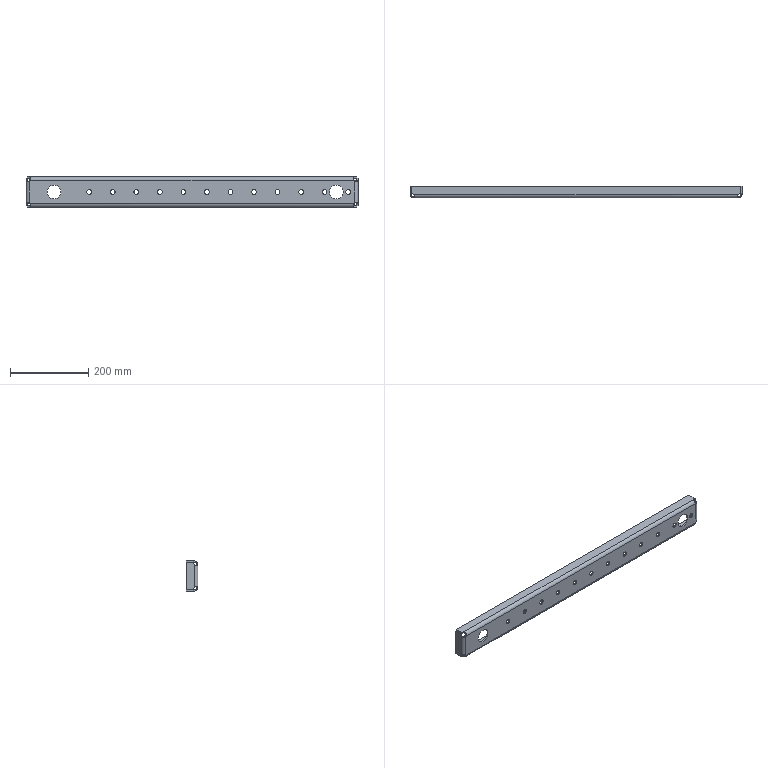Part | SolidWorks | features ICE 2, CornerRelief 1, EdgeFlange 1, FlatPattern 1, LPattern 1, SMBaseFlange 1, SheetMetal 1 | 1 solid | 78 faces | box 846 x 30 x 76.5 mm | volume 333721 mm3 | cylinder 48 | plane 22 | spline 8 | commonest cylinder face diameters 12 x24 16 x12 10 x4 16.4 x4 35 x4